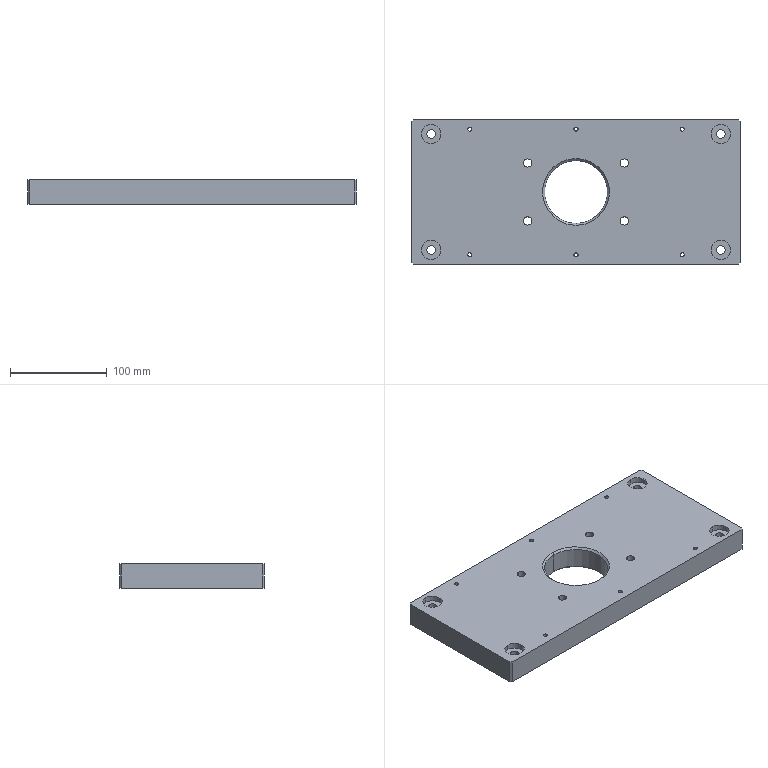CAM job | NX | 3-axis milling, drilling | part box 340 x 150 x 25 mm | stock box 340 x 150 x 25 mm
Tools:
number,name,description,diameter,corner_radius,flute_length,length,flutes
7,D6A45,Milling Tool-5 Parameters,6.0,0.0,3.0,3.0,2
1,ZXZ,Milling Tool-5 Parameters,6.0,0.0,50.0,75.0,2
9,9.0ZT,Drilling Tool,9.0,0.0,35.0,50.0,2
8,8.5ZT,Drilling Tool,8.5,0.0,35.0,50.0,2
14,4.2ZT,Drilling Tool,4.2,0.0,35.0,50.0,2
16,D16R0.8,Milling Tool-5 Parameters,16.0,0.8,50.0,75.0,2
11,D10JING,Milling Tool-5 Parameters,10.0,0.0,50.0,75.0,2
Operations:
program,operation,operation_type,tool,method,geometry_group,spindle_rpm,surface_speed,feed_per_tooth,feed_cut,feed_plunge,cut_length_mm,path_length_mm,cut_time_min,machine_time_min
1,DRILLING_COPY_1,Operation,ZXZ,METHOD,A,3000.0,56.0,0.0333,200.0,0.0,60.0,1088.612,0.3,0.4029
1,DRILLING_COPY_1_COPY_COPY_1_COPY_1,Operation,9.0ZT,METHOD,A,1200.0,33.0,0.05,120.0,0.0,161.019,957.279,1.342,1.421
1,DRILLING_COPY_1_COPY_COPY_1_COPY_1_COPY,Operation,8.5ZT,METHOD,A,1200.0,33.0,0.05,120.0,0.0,128.215,545.624,1.069,1.11
1,DRILLING_COPY_1_COPY_1,Operation,4.2ZT,METHOD,A,2000.0,15.0,0.0375,150.0,0.0,163.571,972.34,1.091,1.171
1,HOLE_MILLING,CylinderMilling,D16R0.8,METHOD,A,2000.0,100.0,0.5,2000.0,100.0,33096.797,33235.297,16.548,16.562
1,HOLE_MILLING_COPY,CylinderMilling,D16R0.8,METHOD,A,2000.0,100.0,0.5,2000.0,100.0,1313.458,2138.568,0.6567,0.7392
1,HOLE_MILLING_1,CylinderMilling,D10JING,METHOD,A,5000.0,157.0,0.085,850.0,100.0,366.607,477.868,0.4313,0.4424
1,ZLEVEL_PROFILE_COPY_1_COPY_COPY_COPY_COPY_2_COPY,ZLevelMilling,D6A45,METHOD,A,4000.0,75.0,0.125,1000.0,1000.0,394.33,3363.088,0.3943,0.6912
1,ZLEVEL_PROFILE_COPY_1_COPY_COPY_COPY_COPY_2_COPY_COPY,ZLevelMilling,D6A45,METHOD,A,4000.0,75.0,0.125,1000.0,1000.0,201.926,266.926,0.2019,0.2084
1,ZLEVEL_PROFILE_COPY_1_COPY_COPY_COPY_COPY_2_COPY_COPY_COPY,ZLevelMilling,D6A45,METHOD,A,4000.0,75.0,0.125,1000.0,1000.0,205.066,270.067,0.2051,0.2116
1,刀补11,CylinderMilling,D10JING,METHOD,A,5000.0,157.0,0.085,850.0,100.0,168.112,1024.089,0.1978,0.2834